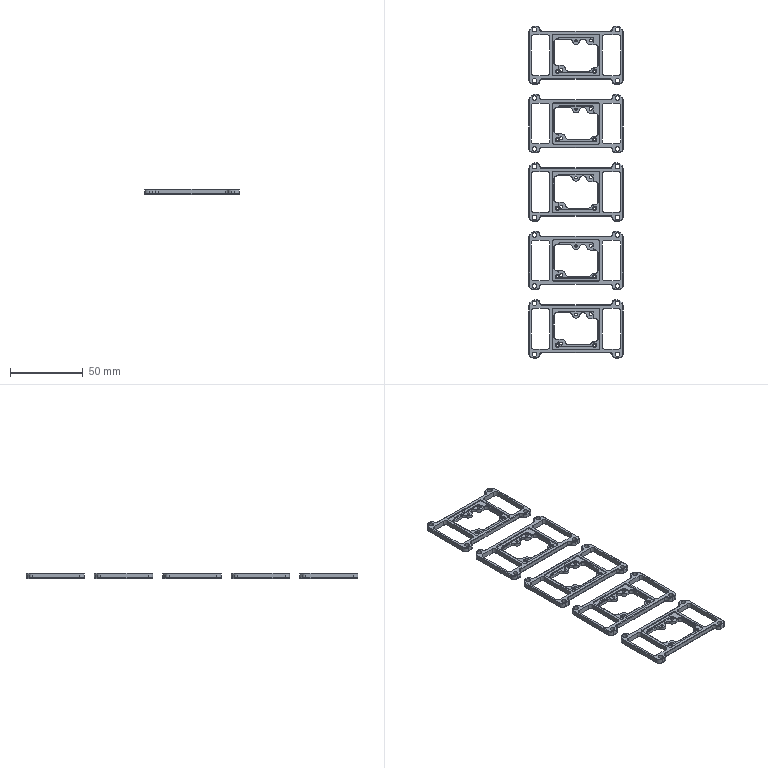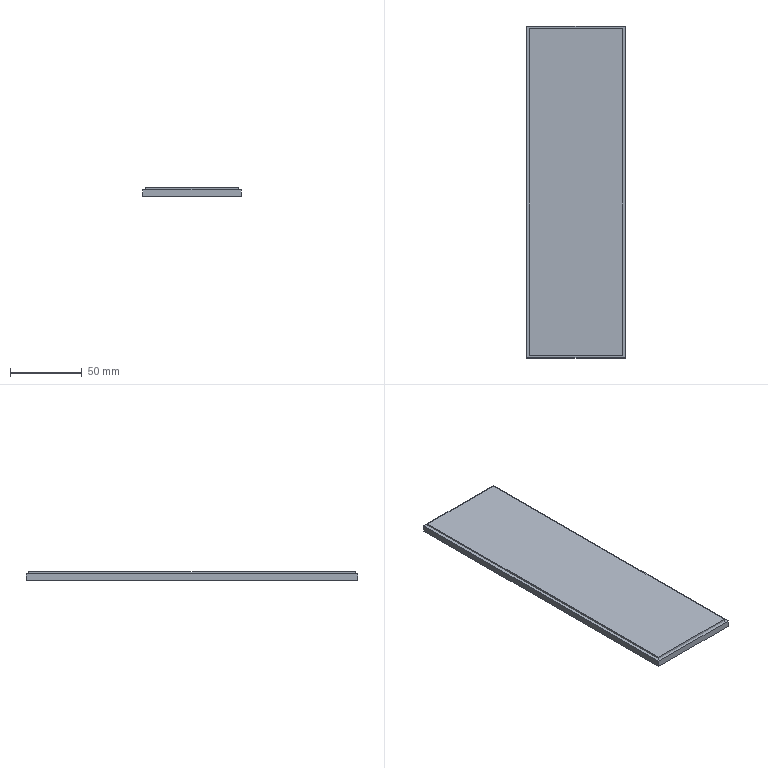CAM job | NX | 3-axis milling | part box 65 x 228 x 3.5 mm | stock box 69 x 232 x 6 mm
Tools:
number,name,description,diameter,corner_radius,flute_length,length,flutes
19,D80,Milling Tool-5 Parameters,80.0,0.0,50.0,75.0,2
12,D6,Milling Tool-5 Parameters,6.0,0.0,50.0,75.0,2
4,D4,Milling Tool-5 Parameters,4.0,0.0,50.0,75.0,2
17,D1.5,Milling Tool-5 Parameters,1.5,0.0,50.0,75.0,2
18,D1,Milling Tool-5 Parameters,1.0,0.0,50.0,75.0,2
1,D6A45,Milling Tool-5 Parameters,6.0,0.0,50.0,75.0,2
Operations:
program,operation,operation_type,tool,method,geometry_group,spindle_rpm,surface_speed,feed_per_tooth,feed_cut,feed_plunge,cut_length_mm,path_length_mm,cut_time_min,machine_time_min
1,FLOOR_WALL,VolumeBased25DMillingOperation,D80,METHOD,A,6500.0,1633.0,0.1154,1500.0,100.0,324.0,378.0,0.216,0.2214
1,ZLEVEL_PROFILE,ZLevelMilling,D6,METHOD,A,9500.0,298.0,0.1579,3000.0,1000.0,15476.185,18650.512,5.689,6.007
1,ZLEVEL_PROFILE_COPY_1,ZLevelMilling,D6,METHOD,A,9500.0,298.0,0.0789,1500.0,1000.0,2158.536,5427.391,1.448,1.775
1,FLOOR_WALL_1,VolumeBased25DMillingOperation,D6,METHOD,A,9500.0,179.0,0.1316,2500.0,100.0,1574.378,2087.457,0.6298,0.6811
1,FLOOR_WALL_1_COPY,VolumeBased25DMillingOperation,D6,METHOD,A,9500.0,179.0,0.1316,2500.0,100.0,1268.466,1744.485,0.5074,0.555
1,FLOOR_WALL_2,VolumeBased25DMillingOperation,D6,METHOD,A,9500.0,179.0,0.0789,1500.0,100.0,2008.11,3008.635,1.339,1.439
1,ZLEVEL_PROFILE_COPY,ZLevelMilling,D4,METHOD,A,9500.0,119.0,0.0789,1500.0,1000.0,5694.986,11912.408,4.362,4.983
1,ZLEVEL_PROFILE_COPY_COPY,ZLevelMilling,D1.5,METHOD,A,9500.0,44.0,0.0526,1000.0,1000.0,7293.997,12470.528,7.294,7.812
1,HOLE_MILLING,CylinderMilling,D1,METHOD,A,9500.0,29.0,0.0447,850.0,100.0,282.178,792.678,0.332,0.383
1,HOLE_MILLING_COPY,CylinderMilling,D1,METHOD,A,9500.0,29.0,0.0447,850.0,100.0,564.356,1526.356,0.6639,0.7601
1,PLANAR_MILL_COPY,PlanarMilling,D6A45,METHOD,A,9500.0,179.0,0.0658,1250.0,100.0,2773.062,5783.202,2.218,2.519
2,FLOOR_WALL_COPY,VolumeBased25DMillingOperation,D80,METHOD,B,6500.0,1633.0,0.1154,1500.0,100.0,960.0,1745.001,0.64,0.7185
2,PLANAR_MILL_COPY_COPY,PlanarMilling,D6A45,METHOD,B,9500.0,179.0,0.0658,1250.0,100.0,2624.578,6410.571,2.1,2.478